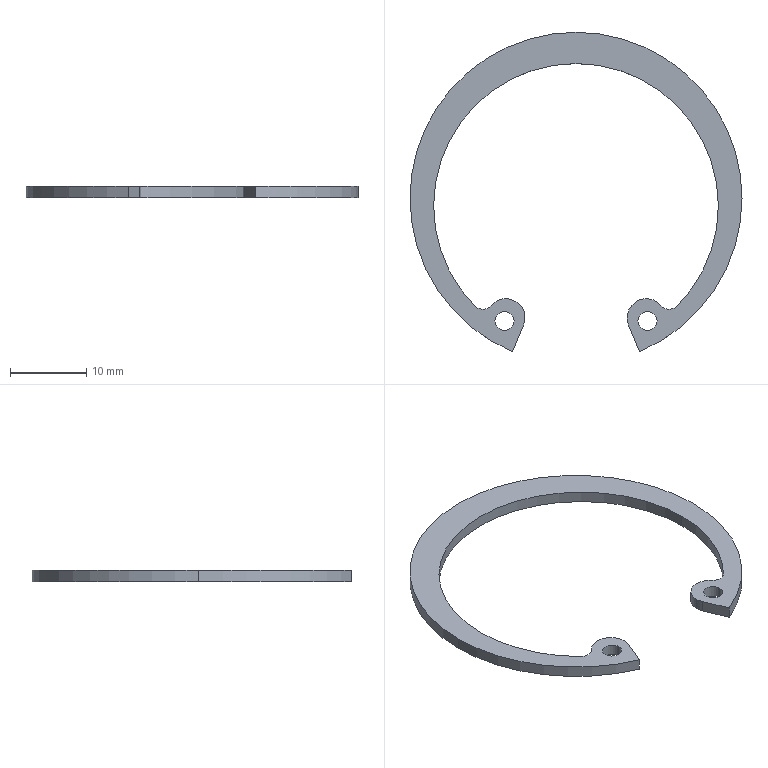Part | SolidWorks | features Extrusion 1 | 1 solid | 19 faces | box 43.5 x 41.844 x 1.5 mm | volume 575.103 mm3 | cylinder 15 | plane 4 | commonest cylinder face diameters 2.5 x4 5 x3 37.3 x3 43.5 x3 3 x2
STEP:
#1=CARTESIAN_POINT('',(8.113,-16.072,0.75));
#2=VERTEX_POINT('',#1);
#3=CARTESIAN_POINT('',(10.613,-16.072,0.75));
#4=VERTEX_POINT('',#3);
#5=CARTESIAN_POINT('',(9.363,-16.072,0.75));
#6=DIRECTION('',(0.,0.,1.));
#7=DIRECTION('',(-1.,0.,0.));
#8=AXIS2_PLACEMENT_3D('',#5,#6,#7);
#9=CIRCLE('',#8,1.25);
#10=EDGE_CURVE('',#2,#4,#9,.T.);
#11=ORIENTED_EDGE('',*,*,#10,.T.);
#12=CARTESIAN_POINT('',(10.613,-16.072,-0.75));
#13=VERTEX_POINT('',#12);
#14=CARTESIAN_POINT('',(10.613,-16.072,0.75));
#15=DIRECTION('',(0.,0.,-1.));
#16=VECTOR('',#15,1000.);
#17=LINE('',#14,#16);
#18=EDGE_CURVE('',#4,#13,#17,.T.);
#19=ORIENTED_EDGE('',*,*,#18,.T.);
#20=CARTESIAN_POINT('',(8.113,-16.072,-0.75));
#21=VERTEX_POINT('',#20);
#22=CARTESIAN_POINT('',(9.363,-16.072,-0.75));
#23=DIRECTION('',(0.,0.,1.));
#24=DIRECTION('',(-1.,0.,0.));
#25=AXIS2_PLACEMENT_3D('',#22,#23,#24);
#26=CIRCLE('',#25,1.25);
#27=EDGE_CURVE('',#21,#13,#26,.T.);
#28=ORIENTED_EDGE('',*,*,#27,.F.);
#29=CARTESIAN_POINT('',(8.113,-16.072,0.75));
#30=DIRECTION('',(0.,0.,-1.));
#31=VECTOR('',#30,1000.);
#32=LINE('',#29,#31);
#33=EDGE_CURVE('',#2,#21,#32,.T.);
#34=ORIENTED_EDGE('',*,*,#33,.F.);
#35=EDGE_LOOP('',(#11,#19,#28,#34));
#36=FACE_OUTER_BOUND('',#35,.T.);
#37=CARTESIAN_POINT('',(9.363,-16.072,0.75));
#38=DIRECTION('',(0.,0.,-1.));
#39=DIRECTION('',(-1.,0.,0.));
#40=AXIS2_PLACEMENT_3D('',#37,#38,#39);
#41=CYLINDRICAL_SURFACE('',#40,1.25);
#42=ADVANCED_FACE('',(#36),#41,.F.);
#43=CARTESIAN_POINT('',(-10.613,-16.072,0.75));
#44=VERTEX_POINT('',#43);
#45=CARTESIAN_POINT('',(-8.113,-16.072,0.75));
#46=VERTEX_POINT('',#45);
#47=CARTESIAN_POINT('',(-9.363,-16.072,0.75));
#48=DIRECTION('',(0.,0.,1.));
#49=DIRECTION('',(1.,0.,0.));
#50=AXIS2_PLACEMENT_3D('',#47,#48,#49);
#51=CIRCLE('',#50,1.25);
#52=EDGE_CURVE('',#44,#46,#51,.T.);
#53=ORIENTED_EDGE('',*,*,#52,.T.);
#54=CARTESIAN_POINT('',(-8.113,-16.072,-0.75));
#55=VERTEX_POINT('',#54);
#56=CARTESIAN_POINT('',(-8.113,-16.072,0.75));
#57=DIRECTION('',(0.,0.,-1.));
#58=VECTOR('',#57,1000.);
#59=LINE('',#56,#58);
#60=EDGE_CURVE('',#46,#55,#59,.T.);
#61=ORIENTED_EDGE('',*,*,#60,.T.);
#62=CARTESIAN_POINT('',(-10.613,-16.072,-0.75));
#63=VERTEX_POINT('',#62);
#64=CARTESIAN_POINT('',(-9.363,-16.072,-0.75));
#65=DIRECTION('',(0.,0.,1.));
#66=DIRECTION('',(1.,0.,0.));
#67=AXIS2_PLACEMENT_3D('',#64,#65,#66);
#68=CIRCLE('',#67,1.25);
#69=EDGE_CURVE('',#63,#55,#68,.T.);
#70=ORIENTED_EDGE('',*,*,#69,.F.);
#71=CARTESIAN_POINT('',(-10.613,-16.072,0.75));
#72=DIRECTION('',(0.,0.,-1.));
#73=VECTOR('',#72,1000.);
#74=LINE('',#71,#73);
#75=EDGE_CURVE('',#44,#63,#74,.T.);
#76=ORIENTED_EDGE('',*,*,#75,.F.);
#77=EDGE_LOOP('',(#53,#61,#70,#76));
#78=FACE_OUTER_BOUND('',#77,.T.);
#79=CARTESIAN_POINT('',(-9.363,-16.072,0.75));
#80=DIRECTION('',(0.,0.,-1.));
#81=DIRECTION('',(-1.,0.,0.));
#82=AXIS2_PLACEMENT_3D('',#79,#80,#81);
#83=CYLINDRICAL_SURFACE('',#82,1.25);
#84=ADVANCED_FACE('',(#78),#83,.F.);
#85=CARTESIAN_POINT('',(21.75,0.,0.75));
#86=VERTEX_POINT('',#85);
#87=CARTESIAN_POINT('',(-21.75,0.,0.75));
#88=VERTEX_POINT('',#87);
#89=CARTESIAN_POINT('',(0.,0.,0.75));
#90=DIRECTION('',(0.,0.,1.));
#91=DIRECTION('',(1.,0.,0.));
#92=AXIS2_PLACEMENT_3D('',#89,#90,#91);
#93=CIRCLE('',#92,21.75);
#94=EDGE_CURVE('',#86,#88,#93,.T.);
#95=ORIENTED_EDGE('',*,*,#94,.F.);
#96=CARTESIAN_POINT('',(21.75,0.,-0.75));
#97=VERTEX_POINT('',#96);
#98=CARTESIAN_POINT('',(21.75,0.,0.75));
#99=DIRECTION('',(0.,0.,-1.));
#100=VECTOR('',#99,1000.);
#101=LINE('',#98,#100);
#102=EDGE_CURVE('',#86,#97,#101,.T.);
#103=ORIENTED_EDGE('',*,*,#102,.T.);
#104=CARTESIAN_POINT('',(-21.75,0.,-0.75));
#105=VERTEX_POINT('',#104);
#106=CARTESIAN_POINT('',(0.,0.,-0.75));
#107=DIRECTION('',(0.,0.,1.));
#108=DIRECTION('',(1.,0.,0.));
#109=AXIS2_PLACEMENT_3D('',#106,#107,#108);
#110=CIRCLE('',#109,21.75);
#111=EDGE_CURVE('',#97,#105,#110,.T.);
#112=ORIENTED_EDGE('',*,*,#111,.T.);
#113=CARTESIAN_POINT('',(-21.75,0.,0.75));
#114=DIRECTION('',(0.,0.,-1.));
#115=VECTOR('',#114,1000.);
#116=LINE('',#113,#115);
#117=EDGE_CURVE('',#88,#105,#116,.T.);
#118=ORIENTED_EDGE('',*,*,#117,.F.);
#119=EDGE_LOOP('',(#95,#103,#112,#118));
#120=FACE_OUTER_BOUND('',#119,.T.);
#121=CARTESIAN_POINT('',(0.,0.,0.75));
#122=DIRECTION('',(0.,0.,-1.));
#123=DIRECTION('',(-1.,0.,0.));
#124=AXIS2_PLACEMENT_3D('',#121,#122,#123);
#125=CYLINDRICAL_SURFACE('',#124,21.75);
#126=ADVANCED_FACE('',(#120),#125,.T.);
#127=CARTESIAN_POINT('',(-8.323,-20.094,0.75));
#128=VERTEX_POINT('',#127);
#129=CARTESIAN_POINT('',(0.,0.,0.75));
#130=DIRECTION('',(0.,0.,1.));
#131=DIRECTION('',(1.,0.,0.));
#132=AXIS2_PLACEMENT_3D('',#129,#130,#131);
#133=CIRCLE('',#132,21.75);
#134=EDGE_CURVE('',#88,#128,#133,.T.);
#135=ORIENTED_EDGE('',*,*,#134,.F.);
#136=ORIENTED_EDGE('',*,*,#117,.T.);
#137=CARTESIAN_POINT('',(-8.323,-20.094,-0.75));
#138=VERTEX_POINT('',#137);
#139=CARTESIAN_POINT('',(0.,0.,-0.75));
#140=DIRECTION('',(0.,0.,1.));
#141=DIRECTION('',(1.,0.,0.));
#142=AXIS2_PLACEMENT_3D('',#139,#140,#141);
#143=CIRCLE('',#142,21.75);
#144=EDGE_CURVE('',#105,#138,#143,.T.);
#145=ORIENTED_EDGE('',*,*,#144,.T.);
#146=CARTESIAN_POINT('',(-8.323,-20.094,0.75));
#147=DIRECTION('',(0.,0.,-1.));
#148=VECTOR('',#147,1000.);
#149=LINE('',#146,#148);
#150=EDGE_CURVE('',#128,#138,#149,.T.);
#151=ORIENTED_EDGE('',*,*,#150,.F.);
#152=EDGE_LOOP('',(#135,#136,#145,#151));
#153=FACE_OUTER_BOUND('',#152,.T.);
#154=CARTESIAN_POINT('',(0.,0.,0.75));
#155=DIRECTION('',(0.,0.,-1.));
#156=DIRECTION('',(-1.,0.,0.));
#157=AXIS2_PLACEMENT_3D('',#154,#155,#156);
#158=CYLINDRICAL_SURFACE('',#157,21.75);
#159=ADVANCED_FACE('',(#153),#158,.T.);
#160=CARTESIAN_POINT('',(6.689,-15.652,0.75));
#161=VERTEX_POINT('',#160);
#162=CARTESIAN_POINT('',(6.879,-16.609,0.75));
#163=VERTEX_POINT('',#162);
#164=CARTESIAN_POINT('',(9.189,-15.652,0.75));
#165=DIRECTION('',(0.,0.,1.));
#166=DIRECTION('',(-1.,0.,0.));
#167=AXIS2_PLACEMENT_3D('',#164,#165,#166);
#168=CIRCLE('',#167,2.5);
#169=EDGE_CURVE('',#161,#163,#168,.T.);
#170=ORIENTED_EDGE('',*,*,#169,.F.);
#171=CARTESIAN_POINT('',(6.689,-15.652,-0.75));
#172=VERTEX_POINT('',#171);
#173=CARTESIAN_POINT('',(6.689,-15.652,0.75));
#174=DIRECTION('',(0.,0.,-1.));
#175=VECTOR('',#174,1000.);
#176=LINE('',#173,#175);
#177=EDGE_CURVE('',#161,#172,#176,.T.);
#178=ORIENTED_EDGE('',*,*,#177,.T.);
#179=CARTESIAN_POINT('',(6.879,-16.609,-0.75));
#180=VERTEX_POINT('',#179);
#181=CARTESIAN_POINT('',(9.189,-15.652,-0.75));
#182=DIRECTION('',(0.,0.,1.));
#183=DIRECTION('',(-1.,0.,0.));
#184=AXIS2_PLACEMENT_3D('',#181,#182,#183);
#185=CIRCLE('',#184,2.5);
#186=EDGE_CURVE('',#172,#180,#185,.T.);
#187=ORIENTED_EDGE('',*,*,#186,.T.);
#188=CARTESIAN_POINT('',(6.879,-16.609,0.75));
#189=DIRECTION('',(0.,0.,-1.));
#190=VECTOR('',#189,1000.);
#191=LINE('',#188,#190);
#192=EDGE_CURVE('',#163,#180,#191,.T.);
#193=ORIENTED_EDGE('',*,*,#192,.F.);
#194=EDGE_LOOP('',(#170,#178,#187,#193));
#195=FACE_OUTER_BOUND('',#194,.T.);
#196=CARTESIAN_POINT('',(9.189,-15.652,0.75));
#197=DIRECTION('',(0.,0.,-1.));
#198=DIRECTION('',(-1.,0.,0.));
#199=AXIS2_PLACEMENT_3D('',#196,#197,#198);
#200=CYLINDRICAL_SURFACE('',#199,2.5);
#201=ADVANCED_FACE('',(#195),#200,.T.);
#202=CARTESIAN_POINT('',(18.65,-1.,0.75));
#203=VERTEX_POINT('',#202);
#204=CARTESIAN_POINT('',(13.285,-14.09,0.75));
#205=VERTEX_POINT('',#204);
#206=CARTESIAN_POINT('',(0.,-1.,0.75));
#207=DIRECTION('',(0.,0.,-1.));
#208=DIRECTION('',(1.,0.,0.));
#209=AXIS2_PLACEMENT_3D('',#206,#207,#208);
#210=CIRCLE('',#209,18.65);
#211=EDGE_CURVE('',#203,#205,#210,.T.);
#212=ORIENTED_EDGE('',*,*,#211,.F.);
#213=CARTESIAN_POINT('',(18.65,-1.,-0.75));
#214=VERTEX_POINT('',#213);
#215=CARTESIAN_POINT('',(18.65,-1.,0.75));
#216=DIRECTION('',(0.,0.,-1.));
#217=VECTOR('',#216,1000.);
#218=LINE('',#215,#217);
#219=EDGE_CURVE('',#203,#214,#218,.T.);
#220=ORIENTED_EDGE('',*,*,#219,.T.);
#221=CARTESIAN_POINT('',(13.285,-14.09,-0.75));
#222=VERTEX_POINT('',#221);
#223=CARTESIAN_POINT('',(0.,-1.,-0.75));
#224=DIRECTION('',(0.,0.,-1.));
#225=DIRECTION('',(1.,0.,0.));
#226=AXIS2_PLACEMENT_3D('',#223,#224,#225);
#227=CIRCLE('',#226,18.65);
#228=EDGE_CURVE('',#214,#222,#227,.T.);
#229=ORIENTED_EDGE('',*,*,#228,.T.);
#230=CARTESIAN_POINT('',(13.285,-14.09,0.75));
#231=DIRECTION('',(0.,0.,-1.));
#232=VECTOR('',#231,1000.);
#233=LINE('',#230,#232);
#234=EDGE_CURVE('',#205,#222,#233,.T.);
#235=ORIENTED_EDGE('',*,*,#234,.F.);
#236=EDGE_LOOP('',(#212,#220,#229,#235));
#237=FACE_OUTER_BOUND('',#236,.T.);
#238=CARTESIAN_POINT('',(0.,-1.,0.75));
#239=DIRECTION('',(0.,0.,-1.));
#240=DIRECTION('',(-1.,0.,0.));
#241=AXIS2_PLACEMENT_3D('',#238,#239,#240);
#242=CYLINDRICAL_SURFACE('',#241,18.65);
#243=ADVANCED_FACE('',(#237),#242,.F.);
#244=ORIENTED_EDGE('',*,*,#219,.F.);
#245=CARTESIAN_POINT('',(-18.65,-1.,0.75));
#246=VERTEX_POINT('',#245);
#247=CARTESIAN_POINT('',(0.,-1.,0.75));
#248=DIRECTION('',(0.,0.,-1.));
#249=DIRECTION('',(1.,0.,0.));
#250=AXIS2_PLACEMENT_3D('',#247,#248,#249);
#251=CIRCLE('',#250,18.65);
#252=EDGE_CURVE('',#246,#203,#251,.T.);
#253=ORIENTED_EDGE('',*,*,#252,.F.);
#254=CARTESIAN_POINT('',(-18.65,-1.,-0.75));
#255=VERTEX_POINT('',#254);
#256=CARTESIAN_POINT('',(-18.65,-1.,0.75));
#257=DIRECTION('',(0.,0.,-1.));
#258=VECTOR('',#257,1000.);
#259=LINE('',#256,#258);
#260=EDGE_CURVE('',#246,#255,#259,.T.);
#261=ORIENTED_EDGE('',*,*,#260,.T.);
#262=CARTESIAN_POINT('',(0.,-1.,-0.75));
#263=DIRECTION('',(0.,0.,-1.));
#264=DIRECTION('',(1.,0.,0.));
#265=AXIS2_PLACEMENT_3D('',#262,#263,#264);
#266=CIRCLE('',#265,18.65);
#267=EDGE_CURVE('',#255,#214,#266,.T.);
#268=ORIENTED_EDGE('',*,*,#267,.T.);
#269=EDGE_LOOP('',(#244,#253,#261,#268));
#270=FACE_OUTER_BOUND('',#269,.T.);
#271=CARTESIAN_POINT('',(0.,-1.,0.75));
#272=DIRECTION('',(0.,0.,-1.));
#273=DIRECTION('',(-1.,0.,0.));
#274=AXIS2_PLACEMENT_3D('',#271,#272,#273);
#275=CYLINDRICAL_SURFACE('',#274,18.65);
#276=ADVANCED_FACE('',(#270),#275,.F.);
#277=ORIENTED_EDGE('',*,*,#52,.F.);
#278=CARTESIAN_POINT('',(-9.363,-16.072,0.75));
#279=DIRECTION('',(0.,0.,1.));
#280=DIRECTION('',(1.,0.,0.));
#281=AXIS2_PLACEMENT_3D('',#278,#279,#280);
#282=CIRCLE('',#281,1.25);
#283=EDGE_CURVE('',#46,#44,#282,.T.);
#284=ORIENTED_EDGE('',*,*,#283,.F.);
#285=EDGE_LOOP('',(#277,#284));
#286=FACE_BOUND('',#285,.T.);
#287=CARTESIAN_POINT('',(-6.879,-16.609,0.75));
#288=VERTEX_POINT('',#287);
#289=CARTESIAN_POINT('',(-11.081,-14.018,0.75));
#290=VERTEX_POINT('',#289);
#291=CARTESIAN_POINT('',(-9.189,-15.652,0.75));
#292=DIRECTION('',(0.,0.,1.));
#293=DIRECTION('',(1.,0.,0.));
#294=AXIS2_PLACEMENT_3D('',#291,#292,#293);
#295=CIRCLE('',#294,2.5);
#296=EDGE_CURVE('',#288,#290,#295,.T.);
#297=ORIENTED_EDGE('',*,*,#296,.T.);
#298=CARTESIAN_POINT('',(-13.285,-14.09,0.75));
#299=VERTEX_POINT('',#298);
#300=CARTESIAN_POINT('',(-12.216,-13.037,0.75));
#301=DIRECTION('',(0.,0.,-1.));
#302=DIRECTION('',(-1.,0.,0.));
#303=AXIS2_PLACEMENT_3D('',#300,#301,#302);
#304=CIRCLE('',#303,1.5);
#305=EDGE_CURVE('',#290,#299,#304,.T.);
#306=ORIENTED_EDGE('',*,*,#305,.T.);
#307=CARTESIAN_POINT('',(0.,-1.,0.75));
#308=DIRECTION('',(0.,0.,-1.));
#309=DIRECTION('',(1.,0.,0.));
#310=AXIS2_PLACEMENT_3D('',#307,#308,#309);
#311=CIRCLE('',#310,18.65);
#312=EDGE_CURVE('',#299,#246,#311,.T.);
#313=ORIENTED_EDGE('',*,*,#312,.T.);
#314=ORIENTED_EDGE('',*,*,#252,.T.);
#315=ORIENTED_EDGE('',*,*,#211,.T.);
#316=CARTESIAN_POINT('',(11.081,-14.018,0.75));
#317=VERTEX_POINT('',#316);
#318=CARTESIAN_POINT('',(12.216,-13.037,0.75));
#319=DIRECTION('',(0.,0.,-1.));
#320=DIRECTION('',(1.,0.,0.));
#321=AXIS2_PLACEMENT_3D('',#318,#319,#320);
#322=CIRCLE('',#321,1.5);
#323=EDGE_CURVE('',#205,#317,#322,.T.);
#324=ORIENTED_EDGE('',*,*,#323,.T.);
#325=CARTESIAN_POINT('',(9.189,-15.652,0.75));
#326=DIRECTION('',(0.,0.,1.));
#327=DIRECTION('',(-1.,0.,0.));
#328=AXIS2_PLACEMENT_3D('',#325,#326,#327);
#329=CIRCLE('',#328,2.5);
#330=EDGE_CURVE('',#317,#161,#329,.T.);
#331=ORIENTED_EDGE('',*,*,#330,.T.);
#332=ORIENTED_EDGE('',*,*,#169,.T.);
#333=CARTESIAN_POINT('',(8.323,-20.094,0.75));
#334=VERTEX_POINT('',#333);
#335=CARTESIAN_POINT('',(6.879,-16.609,0.75));
#336=DIRECTION('',(0.3827,-0.9239,0.));
#337=VECTOR('',#336,1000.);
#338=LINE('',#335,#337);
#339=EDGE_CURVE('',#163,#334,#338,.T.);
#340=ORIENTED_EDGE('',*,*,#339,.T.);
#341=CARTESIAN_POINT('',(0.,0.,0.75));
#342=DIRECTION('',(0.,0.,1.));
#343=DIRECTION('',(1.,0.,0.));
#344=AXIS2_PLACEMENT_3D('',#341,#342,#343);
#345=CIRCLE('',#344,21.75);
#346=EDGE_CURVE('',#334,#86,#345,.T.);
#347=ORIENTED_EDGE('',*,*,#346,.T.);
#348=ORIENTED_EDGE('',*,*,#94,.T.);
#349=ORIENTED_EDGE('',*,*,#134,.T.);
#350=CARTESIAN_POINT('',(-6.879,-16.609,0.75));
#351=DIRECTION('',(0.3827,0.9239,0.));
#352=VECTOR('',#351,1000.);
#353=LINE('',#350,#352);
#354=EDGE_CURVE('',#128,#288,#353,.T.);
#355=ORIENTED_EDGE('',*,*,#354,.T.);
#356=EDGE_LOOP('',(#297,#306,#313,#314,#315,#324,#331,#332,#340,#347,#348,#349,#355));
#357=FACE_OUTER_BOUND('',#356,.T.);
#358=ORIENTED_EDGE('',*,*,#10,.F.);
#359=CARTESIAN_POINT('',(9.363,-16.072,0.75));
#360=DIRECTION('',(0.,0.,1.));
#361=DIRECTION('',(-1.,0.,0.));
#362=AXIS2_PLACEMENT_3D('',#359,#360,#361);
#363=CIRCLE('',#362,1.25);
#364=EDGE_CURVE('',#4,#2,#363,.T.);
#365=ORIENTED_EDGE('',*,*,#364,.F.);
#366=EDGE_LOOP('',(#358,#365));
#367=FACE_BOUND('',#366,.T.);
#368=CARTESIAN_POINT('',(-9.189,-15.652,0.75));
#369=DIRECTION('',(0.,0.,1.));
#370=DIRECTION('',(1.,0.,0.));
#371=AXIS2_PLACEMENT_3D('',#368,#369,#370);
#372=PLANE('',#371);
#373=ADVANCED_FACE('',(#286,#357,#367),#372,.T.);
#374=CARTESIAN_POINT('',(-6.879,-16.609,-0.75));
#375=VERTEX_POINT('',#374);
#376=CARTESIAN_POINT('',(-6.879,-16.609,0.75));
#377=DIRECTION('',(0.,0.,-1.));
#378=VECTOR('',#377,1000.);
#379=LINE('',#376,#378);
#380=EDGE_CURVE('',#288,#375,#379,.T.);
#381=ORIENTED_EDGE('',*,*,#380,.T.);
#382=CARTESIAN_POINT('',(-11.081,-14.018,-0.75));
#383=VERTEX_POINT('',#382);
#384=CARTESIAN_POINT('',(-9.189,-15.652,-0.75));
#385=DIRECTION('',(0.,0.,1.));
#386=DIRECTION('',(1.,0.,0.));
#387=AXIS2_PLACEMENT_3D('',#384,#385,#386);
#388=CIRCLE('',#387,2.5);
#389=EDGE_CURVE('',#375,#383,#388,.T.);
#390=ORIENTED_EDGE('',*,*,#389,.T.);
#391=CARTESIAN_POINT('',(-11.081,-14.018,0.75));
#392=DIRECTION('',(0.,0.,-1.));
#393=VECTOR('',#392,1000.);
#394=LINE('',#391,#393);
#395=EDGE_CURVE('',#290,#383,#394,.T.);
#396=ORIENTED_EDGE('',*,*,#395,.F.);
#397=ORIENTED_EDGE('',*,*,#296,.F.);
#398=EDGE_LOOP('',(#381,#390,#396,#397));
#399=FACE_OUTER_BOUND('',#398,.T.);
#400=CARTESIAN_POINT('',(-9.189,-15.652,0.75));
#401=DIRECTION('',(0.,0.,-1.));
#402=DIRECTION('',(-1.,0.,0.));
#403=AXIS2_PLACEMENT_3D('',#400,#401,#402);
#404=CYLINDRICAL_SURFACE('',#403,2.5);
#405=ADVANCED_FACE('',(#399),#404,.T.);
#406=ORIENTED_EDGE('',*,*,#395,.T.);
#407=CARTESIAN_POINT('',(-13.285,-14.09,-0.75));
#408=VERTEX_POINT('',#407);
#409=CARTESIAN_POINT('',(-12.216,-13.037,-0.75));
#410=DIRECTION('',(0.,0.,-1.));
#411=DIRECTION('',(-1.,0.,0.));
#412=AXIS2_PLACEMENT_3D('',#409,#410,#411);
#413=CIRCLE('',#412,1.5);
#414=EDGE_CURVE('',#383,#408,#413,.T.);
#415=ORIENTED_EDGE('',*,*,#414,.T.);
#416=CARTESIAN_POINT('',(-13.285,-14.09,0.75));
#417=DIRECTION('',(0.,0.,-1.));
#418=VECTOR('',#417,1000.);
#419=LINE('',#416,#418);
#420=EDGE_CURVE('',#299,#408,#419,.T.);
#421=ORIENTED_EDGE('',*,*,#420,.F.);
#422=ORIENTED_EDGE('',*,*,#305,.F.);
#423=EDGE_LOOP('',(#406,#415,#421,#422));
#424=FACE_OUTER_BOUND('',#423,.T.);
#425=CARTESIAN_POINT('',(-12.216,-13.037,0.75));
#426=DIRECTION('',(0.,0.,-1.));
#427=DIRECTION('',(-1.,0.,0.));
#428=AXIS2_PLACEMENT_3D('',#425,#426,#427);
#429=CYLINDRICAL_SURFACE('',#428,1.5);
#430=ADVANCED_FACE('',(#424),#429,.F.);
#431=ORIENTED_EDGE('',*,*,#260,.F.);
#432=ORIENTED_EDGE('',*,*,#312,.F.);
#433=ORIENTED_EDGE('',*,*,#420,.T.);
#434=CARTESIAN_POINT('',(0.,-1.,-0.75));
#435=DIRECTION('',(0.,0.,-1.));
#436=DIRECTION('',(1.,0.,0.));
#437=AXIS2_PLACEMENT_3D('',#434,#435,#436);
#438=CIRCLE('',#437,18.65);
#439=EDGE_CURVE('',#408,#255,#438,.T.);
#440=ORIENTED_EDGE('',*,*,#439,.T.);
#441=EDGE_LOOP('',(#431,#432,#433,#440));
#442=FACE_OUTER_BOUND('',#441,.T.);
#443=CARTESIAN_POINT('',(0.,-1.,0.75));
#444=DIRECTION('',(0.,0.,-1.));
#445=DIRECTION('',(-1.,0.,0.));
#446=AXIS2_PLACEMENT_3D('',#443,#444,#445);
#447=CYLINDRICAL_SURFACE('',#446,18.65);
#448=ADVANCED_FACE('',(#442),#447,.F.);
#449=ORIENTED_EDGE('',*,*,#234,.T.);
#450=CARTESIAN_POINT('',(11.081,-14.018,-0.75));
#451=VERTEX_POINT('',#450);
#452=CARTESIAN_POINT('',(12.216,-13.037,-0.75));
#453=DIRECTION('',(0.,0.,-1.));
#454=DIRECTION('',(1.,0.,0.));
#455=AXIS2_PLACEMENT_3D('',#452,#453,#454);
#456=CIRCLE('',#455,1.5);
#457=EDGE_CURVE('',#222,#451,#456,.T.);
#458=ORIENTED_EDGE('',*,*,#457,.T.);
#459=CARTESIAN_POINT('',(11.081,-14.018,0.75));
#460=DIRECTION('',(0.,0.,-1.));
#461=VECTOR('',#460,1000.);
#462=LINE('',#459,#461);
#463=EDGE_CURVE('',#317,#451,#462,.T.);
#464=ORIENTED_EDGE('',*,*,#463,.F.);
#465=ORIENTED_EDGE('',*,*,#323,.F.);
#466=EDGE_LOOP('',(#449,#458,#464,#465));
#467=FACE_OUTER_BOUND('',#466,.T.);
#468=CARTESIAN_POINT('',(12.216,-13.037,0.75));
#469=DIRECTION('',(0.,0.,-1.));
#470=DIRECTION('',(-1.,0.,0.));
#471=AXIS2_PLACEMENT_3D('',#468,#469,#470);
#472=CYLINDRICAL_SURFACE('',#471,1.5);
#473=ADVANCED_FACE('',(#467),#472,.F.);
#474=ORIENTED_EDGE('',*,*,#177,.F.);
#475=ORIENTED_EDGE('',*,*,#330,.F.);
#476=ORIENTED_EDGE('',*,*,#463,.T.);
#477=CARTESIAN_POINT('',(9.189,-15.652,-0.75));
#478=DIRECTION('',(0.,0.,1.));
#479=DIRECTION('',(-1.,0.,0.));
#480=AXIS2_PLACEMENT_3D('',#477,#478,#479);
#481=CIRCLE('',#480,2.5);
#482=EDGE_CURVE('',#451,#172,#481,.T.);
#483=ORIENTED_EDGE('',*,*,#482,.T.);
#484=EDGE_LOOP('',(#474,#475,#476,#483));
#485=FACE_OUTER_BOUND('',#484,.T.);
#486=CARTESIAN_POINT('',(9.189,-15.652,0.75));
#487=DIRECTION('',(0.,0.,-1.));
#488=DIRECTION('',(-1.,0.,0.));
#489=AXIS2_PLACEMENT_3D('',#486,#487,#488);
#490=CYLINDRICAL_SURFACE('',#489,2.5);
#491=ADVANCED_FACE('',(#485),#490,.T.);
#492=ORIENTED_EDGE('',*,*,#192,.T.);
#493=CARTESIAN_POINT('',(8.323,-20.094,-0.75));
#494=VERTEX_POINT('',#493);
#495=CARTESIAN_POINT('',(6.879,-16.609,-0.75));
#496=DIRECTION('',(0.3827,-0.9239,0.));
#497=VECTOR('',#496,1000.);
#498=LINE('',#495,#497);
#499=EDGE_CURVE('',#180,#494,#498,.T.);
#500=ORIENTED_EDGE('',*,*,#499,.T.);
#501=CARTESIAN_POINT('',(8.323,-20.094,0.75));
#502=DIRECTION('',(0.,0.,-1.));
#503=VECTOR('',#502,1000.);
#504=LINE('',#501,#503);
#505=EDGE_CURVE('',#334,#494,#504,.T.);
#506=ORIENTED_EDGE('',*,*,#505,.F.);
#507=ORIENTED_EDGE('',*,*,#339,.F.);
#508=EDGE_LOOP('',(#492,#500,#506,#507));
#509=FACE_OUTER_BOUND('',#508,.T.);
#510=CARTESIAN_POINT('',(6.879,-16.609,0.75));
#511=DIRECTION('',(0.9239,0.3827,0.));
#512=DIRECTION('',(-0.3827,0.9239,0.));
#513=AXIS2_PLACEMENT_3D('',#510,#511,#512);
#514=PLANE('',#513);
#515=ADVANCED_FACE('',(#509),#514,.F.);
#516=ORIENTED_EDGE('',*,*,#102,.F.);
#517=ORIENTED_EDGE('',*,*,#346,.F.);
#518=ORIENTED_EDGE('',*,*,#505,.T.);
#519=CARTESIAN_POINT('',(0.,0.,-0.75));
#520=DIRECTION('',(0.,0.,1.));
#521=DIRECTION('',(1.,0.,0.));
#522=AXIS2_PLACEMENT_3D('',#519,#520,#521);
#523=CIRCLE('',#522,21.75);
#524=EDGE_CURVE('',#494,#97,#523,.T.);
#525=ORIENTED_EDGE('',*,*,#524,.T.);
#526=EDGE_LOOP('',(#516,#517,#518,#525));
#527=FACE_OUTER_BOUND('',#526,.T.);
#528=CARTESIAN_POINT('',(0.,0.,0.75));
#529=DIRECTION('',(0.,0.,-1.));
#530=DIRECTION('',(-1.,0.,0.));
#531=AXIS2_PLACEMENT_3D('',#528,#529,#530);
#532=CYLINDRICAL_SURFACE('',#531,21.75);
#533=ADVANCED_FACE('',(#527),#532,.T.);
#534=ORIENTED_EDGE('',*,*,#150,.T.);
#535=CARTESIAN_POINT('',(-6.879,-16.609,-0.75));
#536=DIRECTION('',(0.3827,0.9239,0.));
#537=VECTOR('',#536,1000.);
#538=LINE('',#535,#537);
#539=EDGE_CURVE('',#138,#375,#538,.T.);
#540=ORIENTED_EDGE('',*,*,#539,.T.);
#541=ORIENTED_EDGE('',*,*,#380,.F.);
#542=ORIENTED_EDGE('',*,*,#354,.F.);
#543=EDGE_LOOP('',(#534,#540,#541,#542));
#544=FACE_OUTER_BOUND('',#543,.T.);
#545=CARTESIAN_POINT('',(-6.879,-16.609,0.75));
#546=DIRECTION('',(-0.9239,0.3827,0.));
#547=DIRECTION('',(-0.3827,-0.9239,0.));
#548=AXIS2_PLACEMENT_3D('',#545,#546,#547);
#549=PLANE('',#548);
#550=ADVANCED_FACE('',(#544),#549,.F.);
#551=ORIENTED_EDGE('',*,*,#60,.F.);
#552=ORIENTED_EDGE('',*,*,#283,.T.);
#553=ORIENTED_EDGE('',*,*,#75,.T.);
#554=CARTESIAN_POINT('',(-9.363,-16.072,-0.75));
#555=DIRECTION('',(0.,0.,1.));
#556=DIRECTION('',(1.,0.,0.));
#557=AXIS2_PLACEMENT_3D('',#554,#555,#556);
#558=CIRCLE('',#557,1.25);
#559=EDGE_CURVE('',#55,#63,#558,.T.);
#560=ORIENTED_EDGE('',*,*,#559,.F.);
#561=EDGE_LOOP('',(#551,#552,#553,#560));
#562=FACE_OUTER_BOUND('',#561,.T.);
#563=CARTESIAN_POINT('',(-9.363,-16.072,0.75));
#564=DIRECTION('',(0.,0.,-1.));
#565=DIRECTION('',(-1.,0.,0.));
#566=AXIS2_PLACEMENT_3D('',#563,#564,#565);
#567=CYLINDRICAL_SURFACE('',#566,1.25);
#568=ADVANCED_FACE('',(#562),#567,.F.);
#569=ORIENTED_EDGE('',*,*,#18,.F.);
#570=ORIENTED_EDGE('',*,*,#364,.T.);
#571=ORIENTED_EDGE('',*,*,#33,.T.);
#572=CARTESIAN_POINT('',(9.363,-16.072,-0.75));
#573=DIRECTION('',(0.,0.,1.));
#574=DIRECTION('',(-1.,0.,0.));
#575=AXIS2_PLACEMENT_3D('',#572,#573,#574);
#576=CIRCLE('',#575,1.25);
#577=EDGE_CURVE('',#13,#21,#576,.T.);
#578=ORIENTED_EDGE('',*,*,#577,.F.);
#579=EDGE_LOOP('',(#569,#570,#571,#578));
#580=FACE_OUTER_BOUND('',#579,.T.);
#581=CARTESIAN_POINT('',(9.363,-16.072,0.75));
#582=DIRECTION('',(0.,0.,-1.));
#583=DIRECTION('',(-1.,0.,0.));
#584=AXIS2_PLACEMENT_3D('',#581,#582,#583);
#585=CYLINDRICAL_SURFACE('',#584,1.25);
#586=ADVANCED_FACE('',(#580),#585,.F.);
#587=ORIENTED_EDGE('',*,*,#27,.T.);
#588=ORIENTED_EDGE('',*,*,#577,.T.);
#589=EDGE_LOOP('',(#587,#588));
#590=FACE_BOUND('',#589,.T.);
#591=ORIENTED_EDGE('',*,*,#69,.T.);
#592=ORIENTED_EDGE('',*,*,#559,.T.);
#593=EDGE_LOOP('',(#591,#592));
#594=FACE_BOUND('',#593,.T.);
#595=ORIENTED_EDGE('',*,*,#389,.F.);
#596=ORIENTED_EDGE('',*,*,#539,.F.);
#597=ORIENTED_EDGE('',*,*,#144,.F.);
#598=ORIENTED_EDGE('',*,*,#111,.F.);
#599=ORIENTED_EDGE('',*,*,#524,.F.);
#600=ORIENTED_EDGE('',*,*,#499,.F.);
#601=ORIENTED_EDGE('',*,*,#186,.F.);
#602=ORIENTED_EDGE('',*,*,#482,.F.);
#603=ORIENTED_EDGE('',*,*,#457,.F.);
#604=ORIENTED_EDGE('',*,*,#228,.F.);
#605=ORIENTED_EDGE('',*,*,#267,.F.);
#606=ORIENTED_EDGE('',*,*,#439,.F.);
#607=ORIENTED_EDGE('',*,*,#414,.F.);
#608=EDGE_LOOP('',(#595,#596,#597,#598,#599,#600,#601,#602,#603,#604,#605,#606,#607));
#609=FACE_OUTER_BOUND('',#608,.T.);
#610=CARTESIAN_POINT('',(-9.189,-15.652,-0.75));
#611=DIRECTION('',(0.,0.,1.));
#612=DIRECTION('',(1.,0.,0.));
#613=AXIS2_PLACEMENT_3D('',#610,#611,#612);
#614=PLANE('',#613);
#615=ADVANCED_FACE('',(#590,#594,#609),#614,.F.);
#616=CLOSED_SHELL('',(#42,#84,#126,#159,#201,#243,#276,#373,#405,#430,#448,#473,#491,#515,#533,#550,#568,#586,#615));
#617=MANIFOLD_SOLID_BREP('',#616);
#618=CARTESIAN_POINT('',(0.,0.,0.));
#619=DIRECTION('',(0.,0.,1.));
#620=DIRECTION('',(1.,0.,0.));
#621=AXIS2_PLACEMENT_3D('',#618,#619,#620);
#622=(LENGTH_UNIT()NAMED_UNIT(*)SI_UNIT(.MILLI.,.METRE.));
#623=UNCERTAINTY_MEASURE_WITH_UNIT(LENGTH_MEASURE(0.00001),#622,'','');
#624=(NAMED_UNIT(*)PLANE_ANGLE_UNIT()SI_UNIT($,.RADIAN.));
#625=(NAMED_UNIT(*)SI_UNIT($,.STERADIAN.)SOLID_ANGLE_UNIT());
#626=(GEOMETRIC_REPRESENTATION_CONTEXT(3)GLOBAL_UNCERTAINTY_ASSIGNED_CONTEXT((#623))GLOBAL_UNIT_ASSIGNED_CONTEXT((#622,#624,#625))REPRESENTATION_CONTEXT('',''));
#627=ADVANCED_BREP_SHAPE_REPRESENTATION('',(#617,#621),#626);